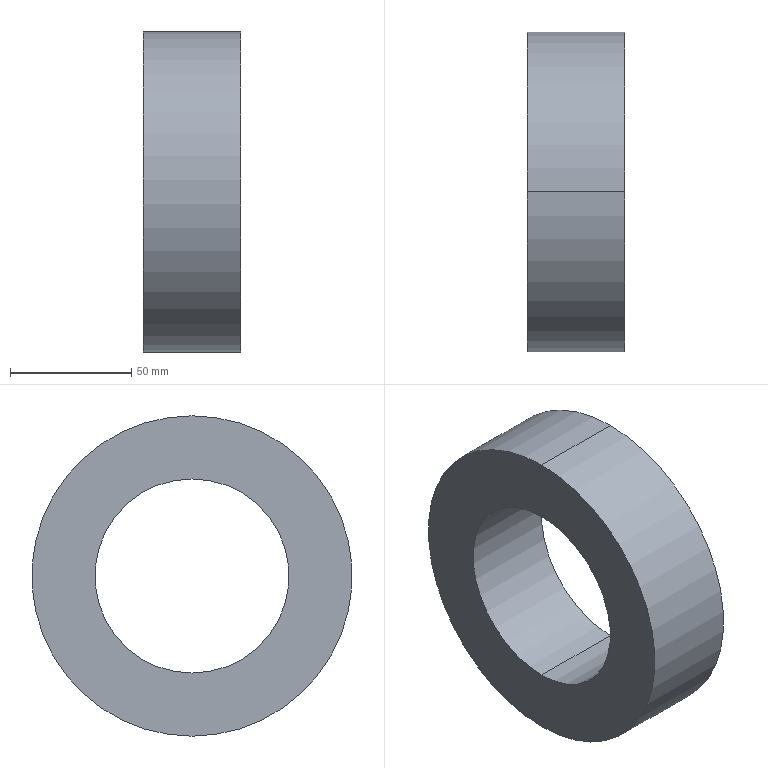Part | NX | features BREP 1 | 1 solid | 6 faces | box 40 x 132 x 132 mm | volume 346329 mm3 | cylinder 4 | plane 2 | commonest cylinder face diameters 80 x2 132 x2
STEP:
#1=CARTESIAN_POINT('',(-310.565,0.,-40.));
#2=VERTEX_POINT('',#1);
#3=CARTESIAN_POINT('',(-310.565,0.,40.));
#4=VERTEX_POINT('',#3);
#5=CARTESIAN_POINT('',(-310.565,0.,0.));
#6=DIRECTION('',(1.,0.,0.));
#7=DIRECTION('',(0.,0.,1.));
#8=AXIS2_PLACEMENT_3D('',#5,#6,#7);
#9=CIRCLE('',#8,40.);
#10=EDGE_CURVE('',#2,#4,#9,.T.);
#11=ORIENTED_EDGE('',*,*,#10,.T.);
#12=CARTESIAN_POINT('',(-350.565,0.,40.));
#13=VERTEX_POINT('',#12);
#14=CARTESIAN_POINT('',(569.435,0.,40.));
#15=DIRECTION('',(-1.,0.,0.));
#16=VECTOR('',#15,1000.);
#17=LINE('',#14,#16);
#18=EDGE_CURVE('',#13,#4,#17,.F.);
#19=ORIENTED_EDGE('',*,*,#18,.F.);
#20=CARTESIAN_POINT('',(-350.565,0.,-40.));
#21=VERTEX_POINT('',#20);
#22=CARTESIAN_POINT('',(-350.565,0.,0.));
#23=DIRECTION('',(-1.,0.,0.));
#24=DIRECTION('',(0.,0.,-1.));
#25=AXIS2_PLACEMENT_3D('',#22,#23,#24);
#26=CIRCLE('',#25,40.);
#27=EDGE_CURVE('',#13,#21,#26,.T.);
#28=ORIENTED_EDGE('',*,*,#27,.T.);
#29=CARTESIAN_POINT('',(569.435,0.,-40.));
#30=DIRECTION('',(-1.,0.,0.));
#31=VECTOR('',#30,1000.);
#32=LINE('',#29,#31);
#33=EDGE_CURVE('',#21,#2,#32,.F.);
#34=ORIENTED_EDGE('',*,*,#33,.T.);
#35=EDGE_LOOP('',(#11,#19,#28,#34));
#36=FACE_BOUND('',#35,.T.);
#37=CARTESIAN_POINT('',(569.435,0.,0.));
#38=DIRECTION('',(-1.,0.,0.));
#39=DIRECTION('',(0.,0.,1.));
#40=AXIS2_PLACEMENT_3D('',#37,#38,#39);
#41=CYLINDRICAL_SURFACE('',#40,40.);
#42=ADVANCED_FACE('',(#36),#41,.F.);
#43=CARTESIAN_POINT('',(-310.565,0.,-66.));
#44=VERTEX_POINT('',#43);
#45=CARTESIAN_POINT('',(-310.565,0.,66.));
#46=VERTEX_POINT('',#45);
#47=CARTESIAN_POINT('',(-310.565,0.,0.));
#48=DIRECTION('',(-1.,0.,0.));
#49=DIRECTION('',(0.,0.,-1.));
#50=AXIS2_PLACEMENT_3D('',#47,#48,#49);
#51=CIRCLE('',#50,66.);
#52=EDGE_CURVE('',#44,#46,#51,.T.);
#53=ORIENTED_EDGE('',*,*,#52,.T.);
#54=CARTESIAN_POINT('',(-350.565,0.,66.));
#55=VERTEX_POINT('',#54);
#56=CARTESIAN_POINT('',(-310.565,0.,66.));
#57=DIRECTION('',(-1.,0.,0.));
#58=VECTOR('',#57,1000.);
#59=LINE('',#56,#58);
#60=EDGE_CURVE('',#55,#46,#59,.F.);
#61=ORIENTED_EDGE('',*,*,#60,.F.);
#62=CARTESIAN_POINT('',(-350.565,0.,-66.));
#63=VERTEX_POINT('',#62);
#64=CARTESIAN_POINT('',(-350.565,0.,0.));
#65=DIRECTION('',(-1.,0.,0.));
#66=DIRECTION('',(0.,0.,-1.));
#67=AXIS2_PLACEMENT_3D('',#64,#65,#66);
#68=CIRCLE('',#67,66.);
#69=EDGE_CURVE('',#63,#55,#68,.T.);
#70=ORIENTED_EDGE('',*,*,#69,.F.);
#71=CARTESIAN_POINT('',(-310.565,0.,-66.));
#72=DIRECTION('',(-1.,0.,0.));
#73=VECTOR('',#72,1000.);
#74=LINE('',#71,#73);
#75=EDGE_CURVE('',#63,#44,#74,.F.);
#76=ORIENTED_EDGE('',*,*,#75,.T.);
#77=EDGE_LOOP('',(#53,#61,#70,#76));
#78=FACE_BOUND('',#77,.T.);
#79=CARTESIAN_POINT('',(-310.565,0.,0.));
#80=DIRECTION('',(-1.,0.,0.));
#81=DIRECTION('',(0.,0.,1.));
#82=AXIS2_PLACEMENT_3D('',#79,#80,#81);
#83=CYLINDRICAL_SURFACE('',#82,66.);
#84=ADVANCED_FACE('',(#78),#83,.T.);
#85=ORIENTED_EDGE('',*,*,#60,.T.);
#86=CARTESIAN_POINT('',(-310.565,0.,0.));
#87=DIRECTION('',(-1.,0.,0.));
#88=DIRECTION('',(0.,0.,-1.));
#89=AXIS2_PLACEMENT_3D('',#86,#87,#88);
#90=CIRCLE('',#89,66.);
#91=EDGE_CURVE('',#46,#44,#90,.T.);
#92=ORIENTED_EDGE('',*,*,#91,.T.);
#93=ORIENTED_EDGE('',*,*,#75,.F.);
#94=CARTESIAN_POINT('',(-350.565,0.,0.));
#95=DIRECTION('',(-1.,0.,0.));
#96=DIRECTION('',(0.,0.,-1.));
#97=AXIS2_PLACEMENT_3D('',#94,#95,#96);
#98=CIRCLE('',#97,66.);
#99=EDGE_CURVE('',#55,#63,#98,.T.);
#100=ORIENTED_EDGE('',*,*,#99,.F.);
#101=EDGE_LOOP('',(#85,#92,#93,#100));
#102=FACE_BOUND('',#101,.T.);
#103=CARTESIAN_POINT('',(-310.565,0.,0.));
#104=DIRECTION('',(-1.,0.,0.));
#105=DIRECTION('',(0.,0.,1.));
#106=AXIS2_PLACEMENT_3D('',#103,#104,#105);
#107=CYLINDRICAL_SURFACE('',#106,66.);
#108=ADVANCED_FACE('',(#102),#107,.T.);
#109=ORIENTED_EDGE('',*,*,#52,.F.);
#110=ORIENTED_EDGE('',*,*,#91,.F.);
#111=EDGE_LOOP('',(#109,#110));
#112=FACE_BOUND('',#111,.T.);
#113=ORIENTED_EDGE('',*,*,#10,.F.);
#114=CARTESIAN_POINT('',(-310.565,0.,0.));
#115=DIRECTION('',(1.,0.,0.));
#116=DIRECTION('',(0.,0.,1.));
#117=AXIS2_PLACEMENT_3D('',#114,#115,#116);
#118=CIRCLE('',#117,40.);
#119=EDGE_CURVE('',#4,#2,#118,.T.);
#120=ORIENTED_EDGE('',*,*,#119,.F.);
#121=EDGE_LOOP('',(#113,#120));
#122=FACE_BOUND('',#121,.T.);
#123=CARTESIAN_POINT('',(-310.565,0.,0.));
#124=DIRECTION('',(1.,0.,0.));
#125=DIRECTION('',(0.,0.,1.));
#126=AXIS2_PLACEMENT_3D('',#123,#124,#125);
#127=PLANE('',#126);
#128=ADVANCED_FACE('',(#112,#122),#127,.T.);
#129=ORIENTED_EDGE('',*,*,#18,.T.);
#130=ORIENTED_EDGE('',*,*,#119,.T.);
#131=ORIENTED_EDGE('',*,*,#33,.F.);
#132=CARTESIAN_POINT('',(-350.565,0.,0.));
#133=DIRECTION('',(-1.,0.,0.));
#134=DIRECTION('',(0.,0.,-1.));
#135=AXIS2_PLACEMENT_3D('',#132,#133,#134);
#136=CIRCLE('',#135,40.);
#137=EDGE_CURVE('',#21,#13,#136,.T.);
#138=ORIENTED_EDGE('',*,*,#137,.T.);
#139=EDGE_LOOP('',(#129,#130,#131,#138));
#140=FACE_BOUND('',#139,.T.);
#141=CARTESIAN_POINT('',(569.435,0.,0.));
#142=DIRECTION('',(-1.,0.,0.));
#143=DIRECTION('',(0.,0.,1.));
#144=AXIS2_PLACEMENT_3D('',#141,#142,#143);
#145=CYLINDRICAL_SURFACE('',#144,40.);
#146=ADVANCED_FACE('',(#140),#145,.F.);
#147=ORIENTED_EDGE('',*,*,#69,.T.);
#148=ORIENTED_EDGE('',*,*,#99,.T.);
#149=EDGE_LOOP('',(#147,#148));
#150=FACE_BOUND('',#149,.T.);
#151=ORIENTED_EDGE('',*,*,#137,.F.);
#152=ORIENTED_EDGE('',*,*,#27,.F.);
#153=EDGE_LOOP('',(#151,#152));
#154=FACE_BOUND('',#153,.T.);
#155=CARTESIAN_POINT('',(-350.565,74.347,-6.052));
#156=DIRECTION('',(1.,0.,0.));
#157=DIRECTION('',(0.,0.,1.));
#158=AXIS2_PLACEMENT_3D('',#155,#156,#157);
#159=PLANE('',#158);
#160=ADVANCED_FACE('',(#150,#154),#159,.F.);
#161=CLOSED_SHELL('',(#42,#84,#108,#128,#146,#160));
#162=MANIFOLD_SOLID_BREP('',#161);
#163=(LENGTH_UNIT()NAMED_UNIT(*)SI_UNIT(.MILLI.,.METRE.));
#164=UNCERTAINTY_MEASURE_WITH_UNIT(LENGTH_MEASURE(0.00001),#163,'','');
#165=(NAMED_UNIT(*)PLANE_ANGLE_UNIT()SI_UNIT($,.RADIAN.));
#166=(NAMED_UNIT(*)SI_UNIT($,.STERADIAN.)SOLID_ANGLE_UNIT());
#167=(GEOMETRIC_REPRESENTATION_CONTEXT(3)GLOBAL_UNCERTAINTY_ASSIGNED_CONTEXT((#164))GLOBAL_UNIT_ASSIGNED_CONTEXT((#163,#165,#166))REPRESENTATION_CONTEXT('',''));
#168=ADVANCED_BREP_SHAPE_REPRESENTATION('',(#162),#167);